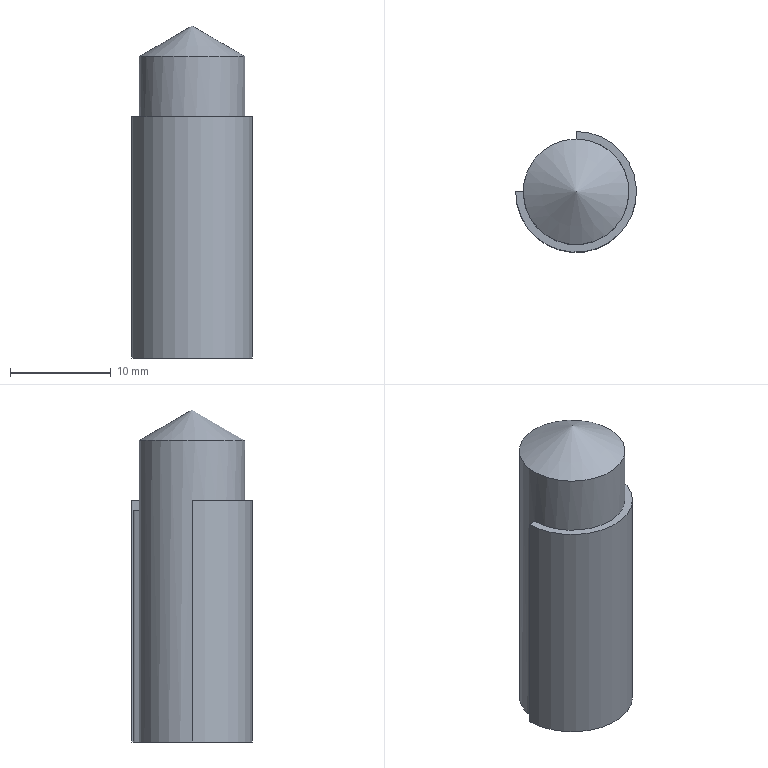Part | NX | features 模具.stp<1>[67] 2 | 1 solid | 10 faces | box 12 x 12 x 32.995 mm | volume 2798 mm3 | plane 6 | cylinder 3 | cone 1 | commonest cylinder face diameters 10.5 x1 11.7 x1 12 x1
STEP:
#1=CARTESIAN_POINT('',(-5.25,-234.,-40.));
#2=VERTEX_POINT('',#1);
#3=CARTESIAN_POINT('',(0.,-234.,-40.));
#4=DIRECTION('',(0.,0.,1.));
#5=DIRECTION('',(-1.,0.,0.));
#6=AXIS2_PLACEMENT_3D('',#3,#4,#5);
#7=CIRCLE('',#6,5.25);
#8=EDGE_CURVE('',#2,#2,#7,.T.);
#9=ORIENTED_EDGE('',*,*,#8,.F.);
#10=EDGE_LOOP('',(#9));
#11=FACE_BOUND('',#10,.T.);
#12=CARTESIAN_POINT('',(0.,-234.,-40.));
#13=DIRECTION('',(0.,0.,-1.));
#14=DIRECTION('',(0.,-1.,0.));
#15=AXIS2_PLACEMENT_3D('',#12,#13,#14);
#16=PLANE('',#15);
#17=ADVANCED_FACE('',(#11),#16,.T.);
#18=CARTESIAN_POINT('',(0.,-234.,-7.005));
#19=VERTEX_POINT('',#18);
#20=VERTEX_LOOP('',#19);
#21=FACE_BOUND('',#20,.T.);
#22=CARTESIAN_POINT('',(0.,-228.75,-10.036));
#23=VERTEX_POINT('',#22);
#24=CARTESIAN_POINT('',(0.,-234.,-10.036));
#25=DIRECTION('',(0.,0.,1.));
#26=DIRECTION('',(0.,1.,0.));
#27=AXIS2_PLACEMENT_3D('',#24,#25,#26);
#28=CIRCLE('',#27,5.25);
#29=EDGE_CURVE('',#23,#23,#28,.T.);
#30=ORIENTED_EDGE('',*,*,#29,.T.);
#31=EDGE_LOOP('',(#30));
#32=FACE_BOUND('',#31,.T.);
#33=CARTESIAN_POINT('',(0.,-234.,-8.005));
#34=DIRECTION('',(0.,0.,-1.));
#35=DIRECTION('',(0.,1.,0.));
#36=AXIS2_PLACEMENT_3D('',#33,#34,#35);
#37=CONICAL_SURFACE('',#36,1.732,1.047);
#38=ADVANCED_FACE('',(#21,#32),#37,.T.);
#39=CARTESIAN_POINT('',(0.,-228.75,-17.));
#40=VERTEX_POINT('',#39);
#41=CARTESIAN_POINT('',(0.,-228.15,-17.));
#42=VERTEX_POINT('',#41);
#43=CARTESIAN_POINT('',(0.,-234.,-17.));
#44=DIRECTION('',(0.,1.,0.));
#45=VECTOR('',#44,1000.);
#46=LINE('',#43,#45);
#47=EDGE_CURVE('',#40,#42,#46,.T.);
#48=ORIENTED_EDGE('',*,*,#47,.T.);
#49=CARTESIAN_POINT('',(-5.85,-234.,-17.));
#50=VERTEX_POINT('',#49);
#51=CARTESIAN_POINT('',(0.,-234.,-17.));
#52=DIRECTION('',(0.,0.,-1.));
#53=DIRECTION('',(0.,1.,0.));
#54=AXIS2_PLACEMENT_3D('',#51,#52,#53);
#55=CIRCLE('',#54,5.85);
#56=EDGE_CURVE('',#42,#50,#55,.T.);
#57=ORIENTED_EDGE('',*,*,#56,.T.);
#58=CARTESIAN_POINT('',(-5.25,-234.,-17.));
#59=VERTEX_POINT('',#58);
#60=CARTESIAN_POINT('',(0.,-234.,-17.));
#61=DIRECTION('',(1.,0.,0.));
#62=VECTOR('',#61,1000.);
#63=LINE('',#60,#62);
#64=EDGE_CURVE('',#50,#59,#63,.T.);
#65=ORIENTED_EDGE('',*,*,#64,.T.);
#66=CARTESIAN_POINT('',(0.,-234.,-17.));
#67=DIRECTION('',(0.,0.,1.));
#68=DIRECTION('',(-1.,0.,0.));
#69=AXIS2_PLACEMENT_3D('',#66,#67,#68);
#70=CIRCLE('',#69,5.25);
#71=EDGE_CURVE('',#59,#40,#70,.T.);
#72=ORIENTED_EDGE('',*,*,#71,.T.);
#73=EDGE_LOOP('',(#48,#57,#65,#72));
#74=FACE_BOUND('',#73,.T.);
#75=CARTESIAN_POINT('',(0.,-234.,-17.));
#76=DIRECTION('',(0.,0.,1.));
#77=DIRECTION('',(1.,0.,0.));
#78=AXIS2_PLACEMENT_3D('',#75,#76,#77);
#79=PLANE('',#78);
#80=ADVANCED_FACE('',(#74),#79,.F.);
#81=CARTESIAN_POINT('',(-5.25,-234.,-16.));
#82=VERTEX_POINT('',#81);
#83=CARTESIAN_POINT('',(0.,-228.75,-16.));
#84=VERTEX_POINT('',#83);
#85=CARTESIAN_POINT('',(0.,-234.,-16.));
#86=DIRECTION('',(0.,0.,1.));
#87=DIRECTION('',(-1.,0.,0.));
#88=AXIS2_PLACEMENT_3D('',#85,#86,#87);
#89=CIRCLE('',#88,5.25);
#90=EDGE_CURVE('',#82,#84,#89,.T.);
#91=ORIENTED_EDGE('',*,*,#90,.F.);
#92=CARTESIAN_POINT('',(-6.,-234.,-16.));
#93=VERTEX_POINT('',#92);
#94=CARTESIAN_POINT('',(-6.,-234.,-16.));
#95=DIRECTION('',(-1.,0.,0.));
#96=VECTOR('',#95,1000.);
#97=LINE('',#94,#96);
#98=EDGE_CURVE('',#82,#93,#97,.T.);
#99=ORIENTED_EDGE('',*,*,#98,.T.);
#100=CARTESIAN_POINT('',(0.,-228.,-16.));
#101=VERTEX_POINT('',#100);
#102=CARTESIAN_POINT('',(0.,-234.,-16.));
#103=DIRECTION('',(0.,0.,-1.));
#104=DIRECTION('',(0.,1.,0.));
#105=AXIS2_PLACEMENT_3D('',#102,#103,#104);
#106=CIRCLE('',#105,6.);
#107=EDGE_CURVE('',#101,#93,#106,.T.);
#108=ORIENTED_EDGE('',*,*,#107,.F.);
#109=CARTESIAN_POINT('',(0.,-228.,-16.));
#110=DIRECTION('',(0.,-1.,0.));
#111=VECTOR('',#110,1000.);
#112=LINE('',#109,#111);
#113=EDGE_CURVE('',#101,#84,#112,.T.);
#114=ORIENTED_EDGE('',*,*,#113,.T.);
#115=EDGE_LOOP('',(#91,#99,#108,#114));
#116=FACE_BOUND('',#115,.T.);
#117=CARTESIAN_POINT('',(0.,-234.,-16.));
#118=DIRECTION('',(0.,0.,1.));
#119=DIRECTION('',(1.,0.,0.));
#120=AXIS2_PLACEMENT_3D('',#117,#118,#119);
#121=PLANE('',#120);
#122=ADVANCED_FACE('',(#116),#121,.T.);
#123=ORIENTED_EDGE('',*,*,#8,.T.);
#124=EDGE_LOOP('',(#123));
#125=FACE_BOUND('',#124,.T.);
#126=ORIENTED_EDGE('',*,*,#29,.F.);
#127=EDGE_LOOP('',(#126));
#128=FACE_BOUND('',#127,.T.);
#129=CARTESIAN_POINT('',(0.,-228.75,-10.036));
#130=DIRECTION('',(0.,0.,1.));
#131=VECTOR('',#130,1000.);
#132=LINE('',#129,#131);
#133=EDGE_CURVE('',#40,#84,#132,.T.);
#134=ORIENTED_EDGE('',*,*,#133,.F.);
#135=ORIENTED_EDGE('',*,*,#71,.F.);
#136=CARTESIAN_POINT('',(-5.25,-234.,-10.036));
#137=DIRECTION('',(0.,0.,-1.));
#138=VECTOR('',#137,1000.);
#139=LINE('',#136,#138);
#140=EDGE_CURVE('',#82,#59,#139,.T.);
#141=ORIENTED_EDGE('',*,*,#140,.F.);
#142=ORIENTED_EDGE('',*,*,#90,.T.);
#143=EDGE_LOOP('',(#134,#135,#141,#142));
#144=FACE_BOUND('',#143,.T.);
#145=CARTESIAN_POINT('',(0.,-234.,-10.036));
#146=DIRECTION('',(0.,0.,-1.));
#147=DIRECTION('',(0.,1.,0.));
#148=AXIS2_PLACEMENT_3D('',#145,#146,#147);
#149=CYLINDRICAL_SURFACE('',#148,5.25);
#150=ADVANCED_FACE('',(#125,#128,#144),#149,.T.);
#151=CARTESIAN_POINT('',(-6.,-234.,-40.));
#152=VERTEX_POINT('',#151);
#153=CARTESIAN_POINT('',(-5.85,-234.,-40.));
#154=VERTEX_POINT('',#153);
#155=CARTESIAN_POINT('',(0.,-234.,-40.));
#156=DIRECTION('',(1.,0.,0.));
#157=VECTOR('',#156,1000.);
#158=LINE('',#155,#157);
#159=EDGE_CURVE('',#152,#154,#158,.T.);
#160=ORIENTED_EDGE('',*,*,#159,.F.);
#161=CARTESIAN_POINT('',(-6.,-234.,-16.));
#162=DIRECTION('',(0.,0.,1.));
#163=VECTOR('',#162,1000.);
#164=LINE('',#161,#163);
#165=EDGE_CURVE('',#152,#93,#164,.T.);
#166=ORIENTED_EDGE('',*,*,#165,.T.);
#167=ORIENTED_EDGE('',*,*,#98,.F.);
#168=ORIENTED_EDGE('',*,*,#140,.T.);
#169=ORIENTED_EDGE('',*,*,#64,.F.);
#170=CARTESIAN_POINT('',(-5.85,-234.,-17.));
#171=DIRECTION('',(0.,0.,1.));
#172=VECTOR('',#171,1000.);
#173=LINE('',#170,#172);
#174=EDGE_CURVE('',#154,#50,#173,.T.);
#175=ORIENTED_EDGE('',*,*,#174,.F.);
#176=EDGE_LOOP('',(#160,#166,#167,#168,#169,#175));
#177=FACE_BOUND('',#176,.T.);
#178=CARTESIAN_POINT('',(-6.,-234.,-16.));
#179=DIRECTION('',(0.,-1.,0.));
#180=DIRECTION('',(-1.,0.,0.));
#181=AXIS2_PLACEMENT_3D('',#178,#179,#180);
#182=PLANE('',#181);
#183=ADVANCED_FACE('',(#177),#182,.F.);
#184=CARTESIAN_POINT('',(0.,-228.15,-40.));
#185=VERTEX_POINT('',#184);
#186=CARTESIAN_POINT('',(0.,-228.,-40.));
#187=VERTEX_POINT('',#186);
#188=CARTESIAN_POINT('',(0.,0.,-40.));
#189=DIRECTION('',(0.,1.,0.));
#190=VECTOR('',#189,1000.);
#191=LINE('',#188,#190);
#192=EDGE_CURVE('',#185,#187,#191,.T.);
#193=ORIENTED_EDGE('',*,*,#192,.F.);
#194=CARTESIAN_POINT('',(0.,-228.15,-17.));
#195=DIRECTION('',(0.,0.,-1.));
#196=VECTOR('',#195,1000.);
#197=LINE('',#194,#196);
#198=EDGE_CURVE('',#42,#185,#197,.T.);
#199=ORIENTED_EDGE('',*,*,#198,.F.);
#200=ORIENTED_EDGE('',*,*,#47,.F.);
#201=ORIENTED_EDGE('',*,*,#133,.T.);
#202=ORIENTED_EDGE('',*,*,#113,.F.);
#203=CARTESIAN_POINT('',(0.,-228.,-16.));
#204=DIRECTION('',(0.,0.,-1.));
#205=VECTOR('',#204,1000.);
#206=LINE('',#203,#205);
#207=EDGE_CURVE('',#101,#187,#206,.T.);
#208=ORIENTED_EDGE('',*,*,#207,.T.);
#209=EDGE_LOOP('',(#193,#199,#200,#201,#202,#208));
#210=FACE_BOUND('',#209,.T.);
#211=CARTESIAN_POINT('',(0.,-228.,-16.));
#212=DIRECTION('',(1.,0.,0.));
#213=DIRECTION('',(0.,-1.,0.));
#214=AXIS2_PLACEMENT_3D('',#211,#212,#213);
#215=PLANE('',#214);
#216=ADVANCED_FACE('',(#210),#215,.F.);
#217=CARTESIAN_POINT('',(0.,-234.,-40.));
#218=DIRECTION('',(0.,0.,1.));
#219=DIRECTION('',(-1.,0.,0.));
#220=AXIS2_PLACEMENT_3D('',#217,#218,#219);
#221=CIRCLE('',#220,5.85);
#222=EDGE_CURVE('',#154,#185,#221,.T.);
#223=ORIENTED_EDGE('',*,*,#222,.F.);
#224=ORIENTED_EDGE('',*,*,#174,.T.);
#225=ORIENTED_EDGE('',*,*,#56,.F.);
#226=ORIENTED_EDGE('',*,*,#198,.T.);
#227=EDGE_LOOP('',(#223,#224,#225,#226));
#228=FACE_BOUND('',#227,.T.);
#229=CARTESIAN_POINT('',(0.,-234.,-17.));
#230=DIRECTION('',(0.,0.,-1.));
#231=DIRECTION('',(0.,1.,0.));
#232=AXIS2_PLACEMENT_3D('',#229,#230,#231);
#233=CYLINDRICAL_SURFACE('',#232,5.85);
#234=ADVANCED_FACE('',(#228),#233,.F.);
#235=ORIENTED_EDGE('',*,*,#107,.T.);
#236=ORIENTED_EDGE('',*,*,#165,.F.);
#237=CARTESIAN_POINT('',(0.,-234.,-40.));
#238=DIRECTION('',(0.,0.,1.));
#239=DIRECTION('',(-1.,0.,0.));
#240=AXIS2_PLACEMENT_3D('',#237,#238,#239);
#241=CIRCLE('',#240,6.);
#242=EDGE_CURVE('',#152,#187,#241,.T.);
#243=ORIENTED_EDGE('',*,*,#242,.T.);
#244=ORIENTED_EDGE('',*,*,#207,.F.);
#245=EDGE_LOOP('',(#235,#236,#243,#244));
#246=FACE_BOUND('',#245,.T.);
#247=CARTESIAN_POINT('',(0.,-234.,-16.));
#248=DIRECTION('',(0.,0.,-1.));
#249=DIRECTION('',(0.,1.,0.));
#250=AXIS2_PLACEMENT_3D('',#247,#248,#249);
#251=CYLINDRICAL_SURFACE('',#250,6.);
#252=ADVANCED_FACE('',(#246),#251,.T.);
#253=ORIENTED_EDGE('',*,*,#242,.F.);
#254=ORIENTED_EDGE('',*,*,#159,.T.);
#255=ORIENTED_EDGE('',*,*,#222,.T.);
#256=ORIENTED_EDGE('',*,*,#192,.T.);
#257=EDGE_LOOP('',(#253,#254,#255,#256));
#258=FACE_BOUND('',#257,.T.);
#259=CARTESIAN_POINT('',(0.,-234.,-40.));
#260=DIRECTION('',(0.,0.,-1.));
#261=DIRECTION('',(0.,-1.,0.));
#262=AXIS2_PLACEMENT_3D('',#259,#260,#261);
#263=PLANE('',#262);
#264=ADVANCED_FACE('',(#258),#263,.T.);
#265=CLOSED_SHELL('',(#17,#38,#80,#122,#150,#183,#216,#234,#252,#264));
#266=MANIFOLD_SOLID_BREP('',#265);
#267=(LENGTH_UNIT()NAMED_UNIT(*)SI_UNIT(.MILLI.,.METRE.));
#268=UNCERTAINTY_MEASURE_WITH_UNIT(LENGTH_MEASURE(0.00001),#267,'','');
#269=(NAMED_UNIT(*)PLANE_ANGLE_UNIT()SI_UNIT($,.RADIAN.));
#270=(NAMED_UNIT(*)SI_UNIT($,.STERADIAN.)SOLID_ANGLE_UNIT());
#271=(GEOMETRIC_REPRESENTATION_CONTEXT(3)GLOBAL_UNCERTAINTY_ASSIGNED_CONTEXT((#268))GLOBAL_UNIT_ASSIGNED_CONTEXT((#267,#269,#270))REPRESENTATION_CONTEXT('',''));
#272=ADVANCED_BREP_SHAPE_REPRESENTATION('',(#266),#271);